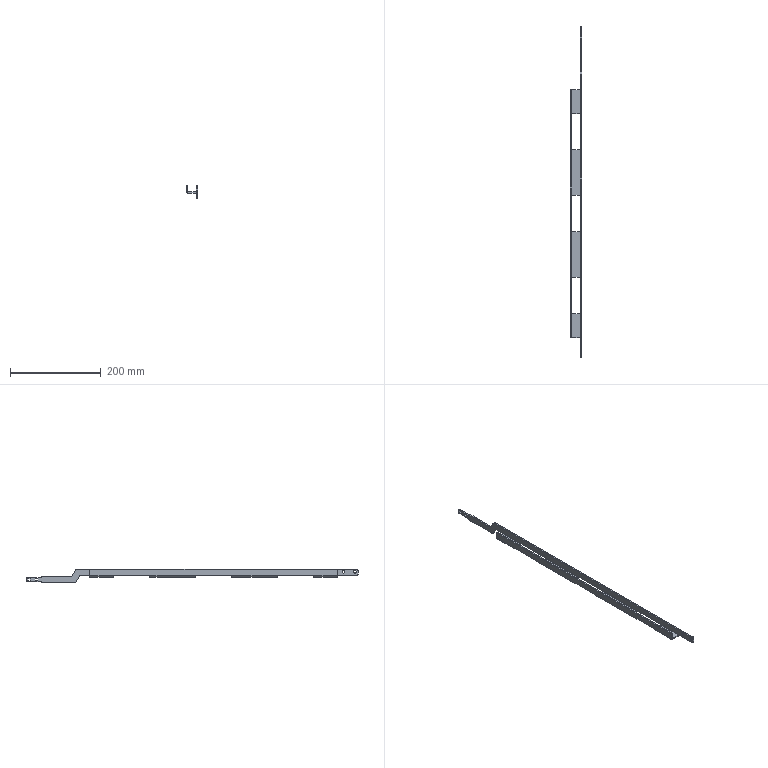Part | SolidWorks | features BaseBody 1 | 1 solid | 85 faces | box 25 x 730 x 30.5 mm | volume 74488 mm3 | plane 57 | cylinder 28 | commonest cylinder face diameters 6 x10 1 x8 7 x8 20 x2